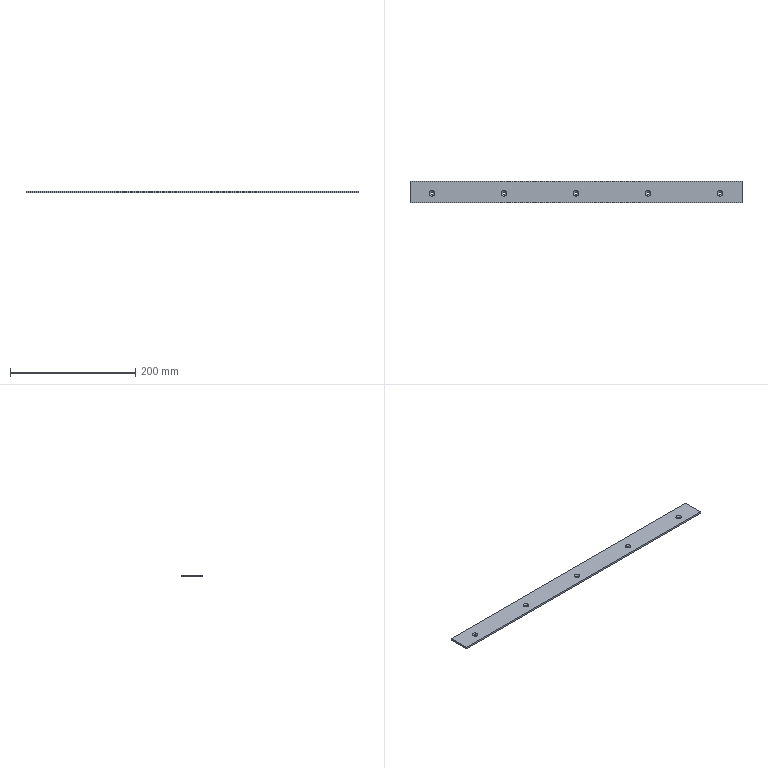Part | STEP file | Belt bracket plate | 1 solid | 26 faces | box 530 x 34 x 3 mm | volume 53588 mm3 | cone 10 | cylinder 10 | plane 6 | commonest cylinder face diameters 4.5 x10